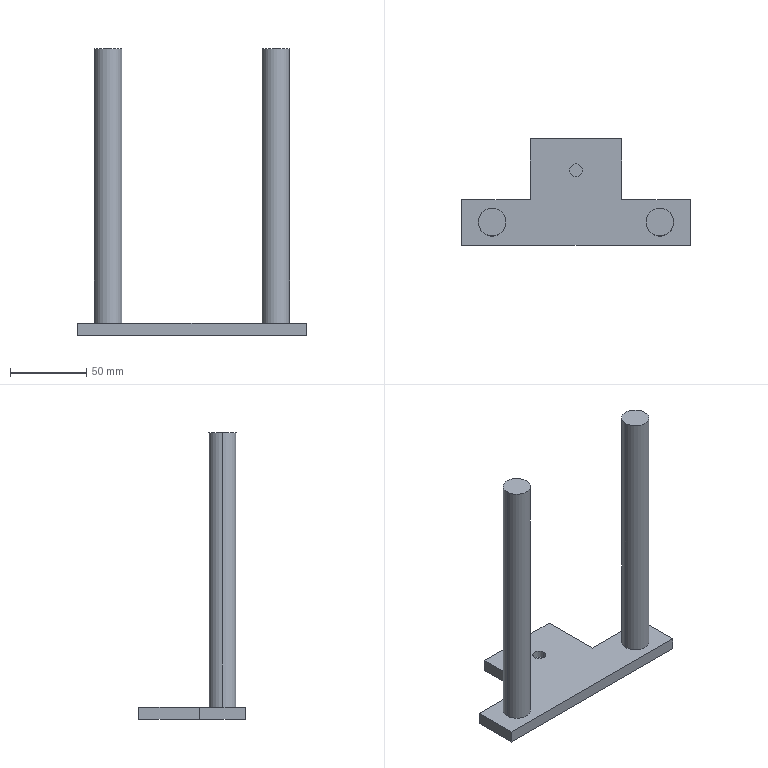Part | STEP file | 1 solid | 19 faces | box 150 x 70 x 188 mm | volume 146525 mm3 | plane 13 | cylinder 6 | commonest cylinder face diameters 18 x4 8.5 x2
STEP:
#1=CARTESIAN_POINT('',(0.,0.,0.));
#2=DIRECTION('',(0.,0.,1.));
#3=DIRECTION('',(1.,0.,0.));
#4=AXIS2_PLACEMENT_3D('',#1,#2,#3);
#5=CARTESIAN_POINT('',(-46.,15.,8.));
#6=VERTEX_POINT('',#5);
#7=CARTESIAN_POINT('',(-64.,15.,8.));
#8=VERTEX_POINT('',#7);
#9=CARTESIAN_POINT('',(-55.,15.,8.));
#10=DIRECTION('',(0.,0.,1.));
#11=DIRECTION('',(1.,0.,0.));
#12=AXIS2_PLACEMENT_3D('',#9,#10,#11);
#13=CIRCLE('',#12,9.);
#14=CARTESIAN_POINT('',(-55.,15.,188.));
#15=DIRECTION('',(0.,0.,1.));
#16=DIRECTION('',(1.,0.,0.));
#17=AXIS2_PLACEMENT_3D('',#14,#15,#16);
#18=CYLINDRICAL_SURFACE('',#17,9.);
#19=CARTESIAN_POINT('',(0.,-180.));
#20=DIRECTION('',(1.,0.));
#21=VECTOR('',#20,1.);
#22=LINE('',#19,#21);
#23=(GEOMETRIC_REPRESENTATION_CONTEXT(2)PARAMETRIC_REPRESENTATION_CONTEXT()REPRESENTATION_CONTEXT('',''));
#24=DEFINITIONAL_REPRESENTATION('',(#22),#23);
#25=PCURVE('',#18,#24);
#26=CARTESIAN_POINT('',(0.,0.,8.));
#27=DIRECTION('',(0.,0.,-1.));
#28=DIRECTION('',(-1.,0.,0.));
#29=AXIS2_PLACEMENT_3D('',#26,#27,#28);
#30=PLANE('',#29);
#31=CARTESIAN_POINT('',(46.,15.));
#32=CARTESIAN_POINT('',(46.,30.588));
#33=CARTESIAN_POINT('',(59.5,22.794));
#34=CARTESIAN_POINT('',(73.,15.));
#35=CARTESIAN_POINT('',(59.5,7.206));
#36=CARTESIAN_POINT('',(46.,-0.5885));
#37=CARTESIAN_POINT('',(46.,15.));
#38=(BOUNDED_CURVE()B_SPLINE_CURVE(2,(#31,#32,#33,#34,#35,#36,#37),.UNSPECIFIED.,.T.,.F.)B_SPLINE_CURVE_WITH_KNOTS((1,2,2,2,2,1),(-2.094,0.,2.094,4.189,6.283,8.378),.UNSPECIFIED.)CURVE()GEOMETRIC_REPRESENTATION_ITEM()RATIONAL_B_SPLINE_CURVE((1.,0.5,1.,0.5,1.,0.5,1.))REPRESENTATION_ITEM(''));
#39=(GEOMETRIC_REPRESENTATION_CONTEXT(2)PARAMETRIC_REPRESENTATION_CONTEXT()REPRESENTATION_CONTEXT('',''));
#40=DEFINITIONAL_REPRESENTATION('',(#38),#39);
#41=PCURVE('',#30,#40);
#42=SURFACE_CURVE('',#13,(#25,#41),.PCURVE_S1.);
#43=EDGE_CURVE('',#6,#8,#42,.T.);
#44=ORIENTED_EDGE('',*,*,#43,.T.);
#45=CARTESIAN_POINT('',(-64.,15.,188.));
#46=VERTEX_POINT('',#45);
#47=CARTESIAN_POINT('',(-64.,15.,188.));
#48=DIRECTION('',(0.,0.,1.));
#49=VECTOR('',#48,1.);
#50=LINE('',#47,#49);
#51=CARTESIAN_POINT('',(3.142,0.));
#52=DIRECTION('',(0.,1.));
#53=VECTOR('',#52,1.);
#54=LINE('',#51,#53);
#55=(GEOMETRIC_REPRESENTATION_CONTEXT(2)PARAMETRIC_REPRESENTATION_CONTEXT()REPRESENTATION_CONTEXT('',''));
#56=DEFINITIONAL_REPRESENTATION('',(#54),#55);
#57=PCURVE('',#18,#56);
#58=CARTESIAN_POINT('',(-55.,15.,188.));
#59=DIRECTION('',(0.,0.,1.));
#60=DIRECTION('',(1.,0.,0.));
#61=AXIS2_PLACEMENT_3D('',#58,#59,#60);
#62=CYLINDRICAL_SURFACE('',#61,9.);
#63=CARTESIAN_POINT('',(3.142,0.));
#64=DIRECTION('',(0.,1.));
#65=VECTOR('',#64,1.);
#66=LINE('',#63,#65);
#67=(GEOMETRIC_REPRESENTATION_CONTEXT(2)PARAMETRIC_REPRESENTATION_CONTEXT()REPRESENTATION_CONTEXT('',''));
#68=DEFINITIONAL_REPRESENTATION('',(#66),#67);
#69=PCURVE('',#62,#68);
#70=SURFACE_CURVE('',#50,(#57,#69),.PCURVE_S1.);
#71=EDGE_CURVE('',#8,#46,#70,.T.);
#72=ORIENTED_EDGE('',*,*,#71,.T.);
#73=CARTESIAN_POINT('',(-46.,15.,188.));
#74=VERTEX_POINT('',#73);
#75=CARTESIAN_POINT('',(-55.,15.,188.));
#76=DIRECTION('',(0.,0.,-1.));
#77=DIRECTION('',(1.,0.,0.));
#78=AXIS2_PLACEMENT_3D('',#75,#76,#77);
#79=CIRCLE('',#78,9.);
#80=CARTESIAN_POINT('',(6.283,0.));
#81=DIRECTION('',(-1.,0.));
#82=VECTOR('',#81,1.);
#83=LINE('',#80,#82);
#84=(GEOMETRIC_REPRESENTATION_CONTEXT(2)PARAMETRIC_REPRESENTATION_CONTEXT()REPRESENTATION_CONTEXT('',''));
#85=DEFINITIONAL_REPRESENTATION('',(#83),#84);
#86=PCURVE('',#18,#85);
#87=CARTESIAN_POINT('',(-55.,15.,188.));
#88=DIRECTION('',(0.,0.,1.));
#89=DIRECTION('',(1.,0.,0.));
#90=AXIS2_PLACEMENT_3D('',#87,#88,#89);
#91=PLANE('',#90);
#92=CARTESIAN_POINT('',(9.,0.));
#93=CARTESIAN_POINT('',(9.,-15.588));
#94=CARTESIAN_POINT('',(-4.5,-7.794));
#95=CARTESIAN_POINT('',(-18.,0.));
#96=CARTESIAN_POINT('',(-4.5,7.794));
#97=CARTESIAN_POINT('',(9.,15.588));
#98=CARTESIAN_POINT('',(9.,0.));
#99=(BOUNDED_CURVE()B_SPLINE_CURVE(2,(#92,#93,#94,#95,#96,#97,#98),.UNSPECIFIED.,.T.,.F.)B_SPLINE_CURVE_WITH_KNOTS((1,2,2,2,2,1),(-2.094,0.,2.094,4.189,6.283,8.378),.UNSPECIFIED.)CURVE()GEOMETRIC_REPRESENTATION_ITEM()RATIONAL_B_SPLINE_CURVE((1.,0.5,1.,0.5,1.,0.5,1.))REPRESENTATION_ITEM(''));
#100=(GEOMETRIC_REPRESENTATION_CONTEXT(2)PARAMETRIC_REPRESENTATION_CONTEXT()REPRESENTATION_CONTEXT('',''));
#101=DEFINITIONAL_REPRESENTATION('',(#99),#100);
#102=PCURVE('',#91,#101);
#103=SURFACE_CURVE('',#79,(#86,#102),.PCURVE_S1.);
#104=EDGE_CURVE('',#46,#74,#103,.T.);
#105=ORIENTED_EDGE('',*,*,#104,.T.);
#106=CARTESIAN_POINT('',(-46.,15.,188.));
#107=DIRECTION('',(0.,0.,1.));
#108=VECTOR('',#107,1.);
#109=LINE('',#106,#108);
#110=CARTESIAN_POINT('',(0.,0.));
#111=DIRECTION('',(0.,1.));
#112=VECTOR('',#111,1.);
#113=LINE('',#110,#112);
#114=(GEOMETRIC_REPRESENTATION_CONTEXT(2)PARAMETRIC_REPRESENTATION_CONTEXT()REPRESENTATION_CONTEXT('',''));
#115=DEFINITIONAL_REPRESENTATION('',(#113),#114);
#116=PCURVE('',#18,#115);
#117=CARTESIAN_POINT('',(6.283,0.));
#118=DIRECTION('',(0.,1.));
#119=VECTOR('',#118,1.);
#120=LINE('',#117,#119);
#121=(GEOMETRIC_REPRESENTATION_CONTEXT(2)PARAMETRIC_REPRESENTATION_CONTEXT()REPRESENTATION_CONTEXT('',''));
#122=DEFINITIONAL_REPRESENTATION('',(#120),#121);
#123=PCURVE('',#62,#122);
#124=SURFACE_CURVE('',#109,(#116,#123),.PCURVE_S1.);
#125=EDGE_CURVE('',#6,#74,#124,.T.);
#126=ORIENTED_EDGE('',*,*,#125,.F.);
#127=EDGE_LOOP('',(#44,#72,#105,#126));
#128=FACE_BOUND('',#127,.T.);
#129=ADVANCED_FACE('',(#128),#18,.T.);
#130=CARTESIAN_POINT('',(64.,15.,8.));
#131=VERTEX_POINT('',#130);
#132=CARTESIAN_POINT('',(46.,15.,8.));
#133=VERTEX_POINT('',#132);
#134=CARTESIAN_POINT('',(55.,15.,8.));
#135=DIRECTION('',(0.,0.,1.));
#136=DIRECTION('',(1.,0.,0.));
#137=AXIS2_PLACEMENT_3D('',#134,#135,#136);
#138=CIRCLE('',#137,9.);
#139=CARTESIAN_POINT('',(55.,15.,188.));
#140=DIRECTION('',(0.,0.,1.));
#141=DIRECTION('',(1.,0.,0.));
#142=AXIS2_PLACEMENT_3D('',#139,#140,#141);
#143=CYLINDRICAL_SURFACE('',#142,9.);
#144=CARTESIAN_POINT('',(0.,-180.));
#145=DIRECTION('',(1.,0.));
#146=VECTOR('',#145,1.);
#147=LINE('',#144,#146);
#148=(GEOMETRIC_REPRESENTATION_CONTEXT(2)PARAMETRIC_REPRESENTATION_CONTEXT()REPRESENTATION_CONTEXT('',''));
#149=DEFINITIONAL_REPRESENTATION('',(#147),#148);
#150=PCURVE('',#143,#149);
#151=CARTESIAN_POINT('',(-64.,15.));
#152=CARTESIAN_POINT('',(-64.,30.588));
#153=CARTESIAN_POINT('',(-50.5,22.794));
#154=CARTESIAN_POINT('',(-37.,15.));
#155=CARTESIAN_POINT('',(-50.5,7.206));
#156=CARTESIAN_POINT('',(-64.,-0.5885));
#157=CARTESIAN_POINT('',(-64.,15.));
#158=(BOUNDED_CURVE()B_SPLINE_CURVE(2,(#151,#152,#153,#154,#155,#156,#157),.UNSPECIFIED.,.T.,.F.)B_SPLINE_CURVE_WITH_KNOTS((1,2,2,2,2,1),(-2.094,0.,2.094,4.189,6.283,8.378),.UNSPECIFIED.)CURVE()GEOMETRIC_REPRESENTATION_ITEM()RATIONAL_B_SPLINE_CURVE((1.,0.5,1.,0.5,1.,0.5,1.))REPRESENTATION_ITEM(''));
#159=(GEOMETRIC_REPRESENTATION_CONTEXT(2)PARAMETRIC_REPRESENTATION_CONTEXT()REPRESENTATION_CONTEXT('',''));
#160=DEFINITIONAL_REPRESENTATION('',(#158),#159);
#161=PCURVE('',#30,#160);
#162=SURFACE_CURVE('',#138,(#150,#161),.PCURVE_S1.);
#163=EDGE_CURVE('',#131,#133,#162,.T.);
#164=ORIENTED_EDGE('',*,*,#163,.T.);
#165=CARTESIAN_POINT('',(46.,15.,188.));
#166=VERTEX_POINT('',#165);
#167=CARTESIAN_POINT('',(46.,15.,188.));
#168=DIRECTION('',(0.,0.,1.));
#169=VECTOR('',#168,1.);
#170=LINE('',#167,#169);
#171=CARTESIAN_POINT('',(3.142,0.));
#172=DIRECTION('',(0.,1.));
#173=VECTOR('',#172,1.);
#174=LINE('',#171,#173);
#175=(GEOMETRIC_REPRESENTATION_CONTEXT(2)PARAMETRIC_REPRESENTATION_CONTEXT()REPRESENTATION_CONTEXT('',''));
#176=DEFINITIONAL_REPRESENTATION('',(#174),#175);
#177=PCURVE('',#143,#176);
#178=CARTESIAN_POINT('',(55.,15.,188.));
#179=DIRECTION('',(0.,0.,1.));
#180=DIRECTION('',(1.,0.,0.));
#181=AXIS2_PLACEMENT_3D('',#178,#179,#180);
#182=CYLINDRICAL_SURFACE('',#181,9.);
#183=CARTESIAN_POINT('',(3.142,0.));
#184=DIRECTION('',(0.,1.));
#185=VECTOR('',#184,1.);
#186=LINE('',#183,#185);
#187=(GEOMETRIC_REPRESENTATION_CONTEXT(2)PARAMETRIC_REPRESENTATION_CONTEXT()REPRESENTATION_CONTEXT('',''));
#188=DEFINITIONAL_REPRESENTATION('',(#186),#187);
#189=PCURVE('',#182,#188);
#190=SURFACE_CURVE('',#170,(#177,#189),.PCURVE_S1.);
#191=EDGE_CURVE('',#133,#166,#190,.T.);
#192=ORIENTED_EDGE('',*,*,#191,.T.);
#193=CARTESIAN_POINT('',(64.,15.,188.));
#194=VERTEX_POINT('',#193);
#195=CARTESIAN_POINT('',(55.,15.,188.));
#196=DIRECTION('',(0.,0.,-1.));
#197=DIRECTION('',(1.,0.,0.));
#198=AXIS2_PLACEMENT_3D('',#195,#196,#197);
#199=CIRCLE('',#198,9.);
#200=CARTESIAN_POINT('',(6.283,0.));
#201=DIRECTION('',(-1.,0.));
#202=VECTOR('',#201,1.);
#203=LINE('',#200,#202);
#204=(GEOMETRIC_REPRESENTATION_CONTEXT(2)PARAMETRIC_REPRESENTATION_CONTEXT()REPRESENTATION_CONTEXT('',''));
#205=DEFINITIONAL_REPRESENTATION('',(#203),#204);
#206=PCURVE('',#143,#205);
#207=CARTESIAN_POINT('',(55.,15.,188.));
#208=DIRECTION('',(0.,0.,-1.));
#209=DIRECTION('',(-1.,0.,0.));
#210=AXIS2_PLACEMENT_3D('',#207,#208,#209);
#211=PLANE('',#210);
#212=CARTESIAN_POINT('',(0.,0.));
#213=DIRECTION('',(-1.,0.));
#214=AXIS2_PLACEMENT_2D('',#212,#213);
#215=CIRCLE('',#214,9.);
#216=(GEOMETRIC_REPRESENTATION_CONTEXT(2)PARAMETRIC_REPRESENTATION_CONTEXT()REPRESENTATION_CONTEXT('',''));
#217=DEFINITIONAL_REPRESENTATION('',(#215),#216);
#218=PCURVE('',#211,#217);
#219=SURFACE_CURVE('',#199,(#206,#218),.PCURVE_S1.);
#220=EDGE_CURVE('',#166,#194,#219,.T.);
#221=ORIENTED_EDGE('',*,*,#220,.T.);
#222=CARTESIAN_POINT('',(64.,15.,188.));
#223=DIRECTION('',(0.,0.,1.));
#224=VECTOR('',#223,1.);
#225=LINE('',#222,#224);
#226=CARTESIAN_POINT('',(0.,0.));
#227=DIRECTION('',(0.,1.));
#228=VECTOR('',#227,1.);
#229=LINE('',#226,#228);
#230=(GEOMETRIC_REPRESENTATION_CONTEXT(2)PARAMETRIC_REPRESENTATION_CONTEXT()REPRESENTATION_CONTEXT('',''));
#231=DEFINITIONAL_REPRESENTATION('',(#229),#230);
#232=PCURVE('',#143,#231);
#233=CARTESIAN_POINT('',(6.283,0.));
#234=DIRECTION('',(0.,1.));
#235=VECTOR('',#234,1.);
#236=LINE('',#233,#235);
#237=(GEOMETRIC_REPRESENTATION_CONTEXT(2)PARAMETRIC_REPRESENTATION_CONTEXT()REPRESENTATION_CONTEXT('',''));
#238=DEFINITIONAL_REPRESENTATION('',(#236),#237);
#239=PCURVE('',#182,#238);
#240=SURFACE_CURVE('',#225,(#232,#239),.PCURVE_S1.);
#241=EDGE_CURVE('',#131,#194,#240,.T.);
#242=ORIENTED_EDGE('',*,*,#241,.F.);
#243=EDGE_LOOP('',(#164,#192,#221,#242));
#244=FACE_BOUND('',#243,.T.);
#245=ADVANCED_FACE('',(#244),#143,.T.);
#246=CARTESIAN_POINT('',(-4.25,49.16,8.));
#247=VERTEX_POINT('',#246);
#248=CARTESIAN_POINT('',(-4.25,49.16,3.));
#249=VERTEX_POINT('',#248);
#250=CARTESIAN_POINT('',(-4.25,49.16,3.));
#251=DIRECTION('',(0.,0.,-1.));
#252=VECTOR('',#251,1.);
#253=LINE('',#250,#252);
#254=CARTESIAN_POINT('',(0.,49.16,3.));
#255=DIRECTION('',(0.,0.,-1.));
#256=DIRECTION('',(-1.,0.,0.));
#257=AXIS2_PLACEMENT_3D('',#254,#255,#256);
#258=CYLINDRICAL_SURFACE('',#257,4.25);
#259=CARTESIAN_POINT('',(6.283,0.));
#260=DIRECTION('',(0.,1.));
#261=VECTOR('',#260,1.);
#262=LINE('',#259,#261);
#263=(GEOMETRIC_REPRESENTATION_CONTEXT(2)PARAMETRIC_REPRESENTATION_CONTEXT()REPRESENTATION_CONTEXT('',''));
#264=DEFINITIONAL_REPRESENTATION('',(#262),#263);
#265=PCURVE('',#258,#264);
#266=CARTESIAN_POINT('',(0.,49.16,3.));
#267=DIRECTION('',(0.,0.,-1.));
#268=DIRECTION('',(-1.,0.,0.));
#269=AXIS2_PLACEMENT_3D('',#266,#267,#268);
#270=CYLINDRICAL_SURFACE('',#269,4.25);
#271=CARTESIAN_POINT('',(0.,0.));
#272=DIRECTION('',(0.,1.));
#273=VECTOR('',#272,1.);
#274=LINE('',#271,#273);
#275=(GEOMETRIC_REPRESENTATION_CONTEXT(2)PARAMETRIC_REPRESENTATION_CONTEXT()REPRESENTATION_CONTEXT('',''));
#276=DEFINITIONAL_REPRESENTATION('',(#274),#275);
#277=PCURVE('',#270,#276);
#278=SURFACE_CURVE('',#253,(#265,#277),.PCURVE_S1.);
#279=EDGE_CURVE('',#247,#249,#278,.T.);
#280=ORIENTED_EDGE('',*,*,#279,.T.);
#281=CARTESIAN_POINT('',(4.25,49.16,3.));
#282=VERTEX_POINT('',#281);
#283=CARTESIAN_POINT('',(0.,49.16,3.));
#284=DIRECTION('',(0.,0.,1.));
#285=DIRECTION('',(-1.,0.,0.));
#286=AXIS2_PLACEMENT_3D('',#283,#284,#285);
#287=CIRCLE('',#286,4.25);
#288=CARTESIAN_POINT('',(6.283,0.));
#289=DIRECTION('',(-1.,0.));
#290=VECTOR('',#289,1.);
#291=LINE('',#288,#290);
#292=(GEOMETRIC_REPRESENTATION_CONTEXT(2)PARAMETRIC_REPRESENTATION_CONTEXT()REPRESENTATION_CONTEXT('',''));
#293=DEFINITIONAL_REPRESENTATION('',(#291),#292);
#294=PCURVE('',#258,#293);
#295=CARTESIAN_POINT('',(0.,49.16,3.));
#296=DIRECTION('',(0.,0.,1.));
#297=DIRECTION('',(1.,0.,0.));
#298=AXIS2_PLACEMENT_3D('',#295,#296,#297);
#299=PLANE('',#298);
#300=CARTESIAN_POINT('',(0.,0.));
#301=DIRECTION('',(-1.,0.));
#302=AXIS2_PLACEMENT_2D('',#300,#301);
#303=CIRCLE('',#302,4.25);
#304=(GEOMETRIC_REPRESENTATION_CONTEXT(2)PARAMETRIC_REPRESENTATION_CONTEXT()REPRESENTATION_CONTEXT('',''));
#305=DEFINITIONAL_REPRESENTATION('',(#303),#304);
#306=PCURVE('',#299,#305);
#307=SURFACE_CURVE('',#287,(#294,#306),.PCURVE_S1.);
#308=EDGE_CURVE('',#249,#282,#307,.T.);
#309=ORIENTED_EDGE('',*,*,#308,.T.);
#310=CARTESIAN_POINT('',(4.25,49.16,8.));
#311=VERTEX_POINT('',#310);
#312=CARTESIAN_POINT('',(4.25,49.16,3.));
#313=DIRECTION('',(0.,0.,-1.));
#314=VECTOR('',#313,1.);
#315=LINE('',#312,#314);
#316=CARTESIAN_POINT('',(3.142,0.));
#317=DIRECTION('',(0.,1.));
#318=VECTOR('',#317,1.);
#319=LINE('',#316,#318);
#320=(GEOMETRIC_REPRESENTATION_CONTEXT(2)PARAMETRIC_REPRESENTATION_CONTEXT()REPRESENTATION_CONTEXT('',''));
#321=DEFINITIONAL_REPRESENTATION('',(#319),#320);
#322=PCURVE('',#258,#321);
#323=CARTESIAN_POINT('',(3.142,0.));
#324=DIRECTION('',(0.,1.));
#325=VECTOR('',#324,1.);
#326=LINE('',#323,#325);
#327=(GEOMETRIC_REPRESENTATION_CONTEXT(2)PARAMETRIC_REPRESENTATION_CONTEXT()REPRESENTATION_CONTEXT('',''));
#328=DEFINITIONAL_REPRESENTATION('',(#326),#327);
#329=PCURVE('',#270,#328);
#330=SURFACE_CURVE('',#315,(#322,#329),.PCURVE_S1.);
#331=EDGE_CURVE('',#311,#282,#330,.T.);
#332=ORIENTED_EDGE('',*,*,#331,.F.);
#333=CARTESIAN_POINT('',(0.,49.16,8.));
#334=DIRECTION('',(0.,0.,1.));
#335=DIRECTION('',(-1.,0.,0.));
#336=AXIS2_PLACEMENT_3D('',#333,#334,#335);
#337=CIRCLE('',#336,4.25);
#338=CARTESIAN_POINT('',(6.283,-5.));
#339=DIRECTION('',(-1.,0.));
#340=VECTOR('',#339,1.);
#341=LINE('',#338,#340);
#342=(GEOMETRIC_REPRESENTATION_CONTEXT(2)PARAMETRIC_REPRESENTATION_CONTEXT()REPRESENTATION_CONTEXT('',''));
#343=DEFINITIONAL_REPRESENTATION('',(#341),#342);
#344=PCURVE('',#258,#343);
#345=CARTESIAN_POINT('',(4.25,49.16));
#346=CARTESIAN_POINT('',(4.25,41.799));
#347=CARTESIAN_POINT('',(-2.125,45.48));
#348=CARTESIAN_POINT('',(-8.5,49.16));
#349=CARTESIAN_POINT('',(-2.125,52.84));
#350=CARTESIAN_POINT('',(4.25,56.521));
#351=CARTESIAN_POINT('',(4.25,49.16));
#352=(BOUNDED_CURVE()B_SPLINE_CURVE(2,(#345,#346,#347,#348,#349,#350,#351),.UNSPECIFIED.,.T.,.F.)B_SPLINE_CURVE_WITH_KNOTS((1,2,2,2,2,1),(-2.094,0.,2.094,4.189,6.283,8.378),.UNSPECIFIED.)CURVE()GEOMETRIC_REPRESENTATION_ITEM()RATIONAL_B_SPLINE_CURVE((1.,0.5,1.,0.5,1.,0.5,1.))REPRESENTATION_ITEM(''));
#353=(GEOMETRIC_REPRESENTATION_CONTEXT(2)PARAMETRIC_REPRESENTATION_CONTEXT()REPRESENTATION_CONTEXT('',''));
#354=DEFINITIONAL_REPRESENTATION('',(#352),#353);
#355=PCURVE('',#30,#354);
#356=SURFACE_CURVE('',#337,(#344,#355),.PCURVE_S1.);
#357=EDGE_CURVE('',#247,#311,#356,.T.);
#358=ORIENTED_EDGE('',*,*,#357,.F.);
#359=EDGE_LOOP('',(#280,#309,#332,#358));
#360=FACE_BOUND('',#359,.F.);
#361=ADVANCED_FACE('',(#360),#258,.F.);
#362=CARTESIAN_POINT('',(-75.,0.,0.));
#363=VERTEX_POINT('',#362);
#364=CARTESIAN_POINT('',(-75.,30.,0.));
#365=VERTEX_POINT('',#364);
#366=CARTESIAN_POINT('',(-75.,0.,0.));
#367=DIRECTION('',(0.,1.,0.));
#368=VECTOR('',#367,1.);
#369=LINE('',#366,#368);
#370=CARTESIAN_POINT('',(0.,0.,0.));
#371=DIRECTION('',(0.,0.,-1.));
#372=DIRECTION('',(-1.,0.,0.));
#373=AXIS2_PLACEMENT_3D('',#370,#371,#372);
#374=PLANE('',#373);
#375=CARTESIAN_POINT('',(75.,0.));
#376=DIRECTION('',(0.,1.));
#377=VECTOR('',#376,1.);
#378=LINE('',#375,#377);
#379=(GEOMETRIC_REPRESENTATION_CONTEXT(2)PARAMETRIC_REPRESENTATION_CONTEXT()REPRESENTATION_CONTEXT('',''));
#380=DEFINITIONAL_REPRESENTATION('',(#378),#379);
#381=PCURVE('',#374,#380);
#382=CARTESIAN_POINT('',(-75.,0.,8.));
#383=DIRECTION('',(1.,0.,0.));
#384=DIRECTION('',(0.,0.,-1.));
#385=AXIS2_PLACEMENT_3D('',#382,#383,#384);
#386=PLANE('',#385);
#387=CARTESIAN_POINT('',(8.,0.));
#388=DIRECTION('',(0.,1.));
#389=VECTOR('',#388,1.);
#390=LINE('',#387,#389);
#391=(GEOMETRIC_REPRESENTATION_CONTEXT(2)PARAMETRIC_REPRESENTATION_CONTEXT()REPRESENTATION_CONTEXT('',''));
#392=DEFINITIONAL_REPRESENTATION('',(#390),#391);
#393=PCURVE('',#386,#392);
#394=SURFACE_CURVE('',#369,(#381,#393),.PCURVE_S1.);
#395=EDGE_CURVE('',#363,#365,#394,.T.);
#396=ORIENTED_EDGE('',*,*,#395,.T.);
#397=CARTESIAN_POINT('',(-30.,30.,0.));
#398=VERTEX_POINT('',#397);
#399=CARTESIAN_POINT('',(0.,30.,0.));
#400=DIRECTION('',(1.,0.,0.));
#401=VECTOR('',#400,1.);
#402=LINE('',#399,#401);
#403=CARTESIAN_POINT('',(0.,30.));
#404=DIRECTION('',(-1.,0.));
#405=VECTOR('',#404,1.);
#406=LINE('',#403,#405);
#407=(GEOMETRIC_REPRESENTATION_CONTEXT(2)PARAMETRIC_REPRESENTATION_CONTEXT()REPRESENTATION_CONTEXT('',''));
#408=DEFINITIONAL_REPRESENTATION('',(#406),#407);
#409=PCURVE('',#374,#408);
#410=CARTESIAN_POINT('',(-75.,30.,8.));
#411=DIRECTION('',(0.,-1.,0.));
#412=DIRECTION('',(0.,0.,-1.));
#413=AXIS2_PLACEMENT_3D('',#410,#411,#412);
#414=PLANE('',#413);
#415=CARTESIAN_POINT('',(8.,75.));
#416=DIRECTION('',(0.,1.));
#417=VECTOR('',#416,1.);
#418=LINE('',#415,#417);
#419=(GEOMETRIC_REPRESENTATION_CONTEXT(2)PARAMETRIC_REPRESENTATION_CONTEXT()REPRESENTATION_CONTEXT('',''));
#420=DEFINITIONAL_REPRESENTATION('',(#418),#419);
#421=PCURVE('',#414,#420);
#422=SURFACE_CURVE('',#402,(#409,#421),.PCURVE_S1.);
#423=EDGE_CURVE('',#365,#398,#422,.T.);
#424=ORIENTED_EDGE('',*,*,#423,.T.);
#425=CARTESIAN_POINT('',(-30.,70.,0.));
#426=VERTEX_POINT('',#425);
#427=CARTESIAN_POINT('',(-30.,0.,0.));
#428=DIRECTION('',(0.,1.,0.));
#429=VECTOR('',#428,1.);
#430=LINE('',#427,#429);
#431=CARTESIAN_POINT('',(30.,0.));
#432=DIRECTION('',(0.,1.));
#433=VECTOR('',#432,1.);
#434=LINE('',#431,#433);
#435=(GEOMETRIC_REPRESENTATION_CONTEXT(2)PARAMETRIC_REPRESENTATION_CONTEXT()REPRESENTATION_CONTEXT('',''));
#436=DEFINITIONAL_REPRESENTATION('',(#434),#435);
#437=PCURVE('',#374,#436);
#438=CARTESIAN_POINT('',(-30.,30.,8.));
#439=DIRECTION('',(1.,0.,0.));
#440=DIRECTION('',(0.,0.,-1.));
#441=AXIS2_PLACEMENT_3D('',#438,#439,#440);
#442=PLANE('',#441);
#443=CARTESIAN_POINT('',(8.,-30.));
#444=DIRECTION('',(0.,1.));
#445=VECTOR('',#444,1.);
#446=LINE('',#443,#445);
#447=(GEOMETRIC_REPRESENTATION_CONTEXT(2)PARAMETRIC_REPRESENTATION_CONTEXT()REPRESENTATION_CONTEXT('',''));
#448=DEFINITIONAL_REPRESENTATION('',(#446),#447);
#449=PCURVE('',#442,#448);
#450=SURFACE_CURVE('',#430,(#437,#449),.PCURVE_S1.);
#451=EDGE_CURVE('',#398,#426,#450,.T.);
#452=ORIENTED_EDGE('',*,*,#451,.T.);
#453=CARTESIAN_POINT('',(30.,70.,0.));
#454=VERTEX_POINT('',#453);
#455=CARTESIAN_POINT('',(0.,70.,0.));
#456=DIRECTION('',(1.,0.,0.));
#457=VECTOR('',#456,1.);
#458=LINE('',#455,#457);
#459=CARTESIAN_POINT('',(0.,70.));
#460=DIRECTION('',(-1.,0.));
#461=VECTOR('',#460,1.);
#462=LINE('',#459,#461);
#463=(GEOMETRIC_REPRESENTATION_CONTEXT(2)PARAMETRIC_REPRESENTATION_CONTEXT()REPRESENTATION_CONTEXT('',''));
#464=DEFINITIONAL_REPRESENTATION('',(#462),#463);
#465=PCURVE('',#374,#464);
#466=CARTESIAN_POINT('',(-30.,70.,8.));
#467=DIRECTION('',(0.,-1.,0.));
#468=DIRECTION('',(1.,0.,0.));
#469=AXIS2_PLACEMENT_3D('',#466,#467,#468);
#470=PLANE('',#469);
#471=CARTESIAN_POINT('',(30.,-8.));
#472=DIRECTION('',(1.,0.));
#473=VECTOR('',#472,1.);
#474=LINE('',#471,#473);
#475=(GEOMETRIC_REPRESENTATION_CONTEXT(2)PARAMETRIC_REPRESENTATION_CONTEXT()REPRESENTATION_CONTEXT('',''));
#476=DEFINITIONAL_REPRESENTATION('',(#474),#475);
#477=PCURVE('',#470,#476);
#478=SURFACE_CURVE('',#458,(#465,#477),.PCURVE_S1.);
#479=EDGE_CURVE('',#426,#454,#478,.T.);
#480=ORIENTED_EDGE('',*,*,#479,.T.);
#481=CARTESIAN_POINT('',(30.,30.,0.));
#482=VERTEX_POINT('',#481);
#483=CARTESIAN_POINT('',(30.,0.,0.));
#484=DIRECTION('',(0.,-1.,0.));
#485=VECTOR('',#484,1.);
#486=LINE('',#483,#485);
#487=CARTESIAN_POINT('',(-30.,0.));
#488=DIRECTION('',(0.,-1.));
#489=VECTOR('',#488,1.);
#490=LINE('',#487,#489);
#491=(GEOMETRIC_REPRESENTATION_CONTEXT(2)PARAMETRIC_REPRESENTATION_CONTEXT()REPRESENTATION_CONTEXT('',''));
#492=DEFINITIONAL_REPRESENTATION('',(#490),#491);
#493=PCURVE('',#374,#492);
#494=CARTESIAN_POINT('',(30.,30.,8.));
#495=DIRECTION('',(-1.,0.,0.));
#496=DIRECTION('',(0.,-1.,0.));
#497=AXIS2_PLACEMENT_3D('',#494,#495,#496);
#498=PLANE('',#497);
#499=CARTESIAN_POINT('',(30.,-8.));
#500=DIRECTION('',(1.,0.));
#501=VECTOR('',#500,1.);
#502=LINE('',#499,#501);
#503=(GEOMETRIC_REPRESENTATION_CONTEXT(2)PARAMETRIC_REPRESENTATION_CONTEXT()REPRESENTATION_CONTEXT('',''));
#504=DEFINITIONAL_REPRESENTATION('',(#502),#503);
#505=PCURVE('',#498,#504);
#506=SURFACE_CURVE('',#486,(#493,#505),.PCURVE_S1.);
#507=EDGE_CURVE('',#454,#482,#506,.T.);
#508=ORIENTED_EDGE('',*,*,#507,.T.);
#509=CARTESIAN_POINT('',(75.,30.,0.));
#510=VERTEX_POINT('',#509);
#511=CARTESIAN_POINT('',(0.,30.,0.));
#512=DIRECTION('',(1.,0.,0.));
#513=VECTOR('',#512,1.);
#514=LINE('',#511,#513);
#515=CARTESIAN_POINT('',(0.,30.));
#516=DIRECTION('',(-1.,0.));
#517=VECTOR('',#516,1.);
#518=LINE('',#515,#517);
#519=(GEOMETRIC_REPRESENTATION_CONTEXT(2)PARAMETRIC_REPRESENTATION_CONTEXT()REPRESENTATION_CONTEXT('',''));
#520=DEFINITIONAL_REPRESENTATION('',(#518),#519);
#521=PCURVE('',#374,#520);
#522=CARTESIAN_POINT('',(75.,30.,8.));
#523=DIRECTION('',(0.,-1.,0.));
#524=DIRECTION('',(1.,0.,0.));
#525=AXIS2_PLACEMENT_3D('',#522,#523,#524);
#526=PLANE('',#525);
#527=CARTESIAN_POINT('',(-75.,-8.));
#528=DIRECTION('',(1.,0.));
#529=VECTOR('',#528,1.);
#530=LINE('',#527,#529);
#531=(GEOMETRIC_REPRESENTATION_CONTEXT(2)PARAMETRIC_REPRESENTATION_CONTEXT()REPRESENTATION_CONTEXT('',''));
#532=DEFINITIONAL_REPRESENTATION('',(#530),#531);
#533=PCURVE('',#526,#532);
#534=SURFACE_CURVE('',#514,(#521,#533),.PCURVE_S1.);
#535=EDGE_CURVE('',#482,#510,#534,.T.);
#536=ORIENTED_EDGE('',*,*,#535,.T.);
#537=CARTESIAN_POINT('',(75.,0.,0.));
#538=VERTEX_POINT('',#537);
#539=CARTESIAN_POINT('',(75.,0.,0.));
#540=DIRECTION('',(0.,-1.,0.));
#541=VECTOR('',#540,1.);
#542=LINE('',#539,#541);
#543=CARTESIAN_POINT('',(-75.,0.));
#544=DIRECTION('',(0.,-1.));
#545=VECTOR('',#544,1.);
#546=LINE('',#543,#545);
#547=(GEOMETRIC_REPRESENTATION_CONTEXT(2)PARAMETRIC_REPRESENTATION_CONTEXT()REPRESENTATION_CONTEXT('',''));
#548=DEFINITIONAL_REPRESENTATION('',(#546),#547);
#549=PCURVE('',#374,#548);
#550=CARTESIAN_POINT('',(75.,0.,8.));
#551=DIRECTION('',(-1.,0.,0.));
#552=DIRECTION('',(0.,0.,1.));
#553=AXIS2_PLACEMENT_3D('',#550,#551,#552);
#554=PLANE('',#553);
#555=CARTESIAN_POINT('',(-8.,0.));
#556=DIRECTION('',(0.,-1.));
#557=VECTOR('',#556,1.);
#558=LINE('',#555,#557);
#559=(GEOMETRIC_REPRESENTATION_CONTEXT(2)PARAMETRIC_REPRESENTATION_CONTEXT()REPRESENTATION_CONTEXT('',''));
#560=DEFINITIONAL_REPRESENTATION('',(#558),#559);
#561=PCURVE('',#554,#560);
#562=SURFACE_CURVE('',#542,(#549,#561),.PCURVE_S1.);
#563=EDGE_CURVE('',#510,#538,#562,.T.);
#564=ORIENTED_EDGE('',*,*,#563,.T.);
#565=CARTESIAN_POINT('',(0.,0.,0.));
#566=DIRECTION('',(-1.,0.,0.));
#567=VECTOR('',#566,1.);
#568=LINE('',#565,#567);
#569=CARTESIAN_POINT('',(0.,0.));
#570=DIRECTION('',(1.,0.));
#571=VECTOR('',#570,1.);
#572=LINE('',#569,#571);
#573=(GEOMETRIC_REPRESENTATION_CONTEXT(2)PARAMETRIC_REPRESENTATION_CONTEXT()REPRESENTATION_CONTEXT('',''));
#574=DEFINITIONAL_REPRESENTATION('',(#572),#573);
#575=PCURVE('',#374,#574);
#576=CARTESIAN_POINT('',(75.,0.,8.));
#577=DIRECTION('',(0.,1.,0.));
#578=DIRECTION('',(-1.,0.,0.));
#579=AXIS2_PLACEMENT_3D('',#576,#577,#578);
#580=PLANE('',#579);
#581=CARTESIAN_POINT('',(75.,-8.));
#582=DIRECTION('',(1.,0.));
#583=VECTOR('',#582,1.);
#584=LINE('',#581,#583);
#585=(GEOMETRIC_REPRESENTATION_CONTEXT(2)PARAMETRIC_REPRESENTATION_CONTEXT()REPRESENTATION_CONTEXT('',''));
#586=DEFINITIONAL_REPRESENTATION('',(#584),#585);
#587=PCURVE('',#580,#586);
#588=SURFACE_CURVE('',#568,(#575,#587),.PCURVE_S1.);
#589=EDGE_CURVE('',#538,#363,#588,.T.);
#590=ORIENTED_EDGE('',*,*,#589,.T.);
#591=EDGE_LOOP('',(#396,#424,#452,#480,#508,#536,#564,#590));
#592=FACE_BOUND('',#591,.T.);
#593=ADVANCED_FACE('',(#592),#374,.T.);
#594=CARTESIAN_POINT('',(-75.,30.,8.));
#595=VERTEX_POINT('',#594);
#596=CARTESIAN_POINT('',(-75.,30.,8.));
#597=DIRECTION('',(0.,0.,-1.));
#598=VECTOR('',#597,1.);
#599=LINE('',#596,#598);
#600=CARTESIAN_POINT('',(0.,0.));
#601=DIRECTION('',(1.,0.));
#602=VECTOR('',#601,1.);
#603=LINE('',#600,#602);
#604=(GEOMETRIC_REPRESENTATION_CONTEXT(2)PARAMETRIC_REPRESENTATION_CONTEXT()REPRESENTATION_CONTEXT('',''));
#605=DEFINITIONAL_REPRESENTATION('',(#603),#604);
#606=PCURVE('',#414,#605);
#607=CARTESIAN_POINT('',(0.,30.));
#608=DIRECTION('',(1.,0.));
#609=VECTOR('',#608,1.);
#610=LINE('',#607,#609);
#611=(GEOMETRIC_REPRESENTATION_CONTEXT(2)PARAMETRIC_REPRESENTATION_CONTEXT()REPRESENTATION_CONTEXT('',''));
#612=DEFINITIONAL_REPRESENTATION('',(#610),#611);
#613=PCURVE('',#386,#612);
#614=SURFACE_CURVE('',#599,(#606,#613),.PCURVE_S1.);
#615=EDGE_CURVE('',#595,#365,#614,.T.);
#616=ORIENTED_EDGE('',*,*,#615,.F.);
#617=CARTESIAN_POINT('',(-30.,30.,8.));
#618=VERTEX_POINT('',#617);
#619=CARTESIAN_POINT('',(-75.,30.,8.));
#620=DIRECTION('',(-1.,0.,0.));
#621=VECTOR('',#620,1.);
#622=LINE('',#619,#621);
#623=CARTESIAN_POINT('',(0.,0.));
#624=DIRECTION('',(0.,-1.));
#625=VECTOR('',#624,1.);
#626=LINE('',#623,#625);
#627=(GEOMETRIC_REPRESENTATION_CONTEXT(2)PARAMETRIC_REPRESENTATION_CONTEXT()REPRESENTATION_CONTEXT('',''));
#628=DEFINITIONAL_REPRESENTATION('',(#626),#627);
#629=PCURVE('',#414,#628);
#630=CARTESIAN_POINT('',(75.,30.));
#631=DIRECTION('',(1.,0.));
#632=VECTOR('',#631,1.);
#633=LINE('',#630,#632);
#634=(GEOMETRIC_REPRESENTATION_CONTEXT(2)PARAMETRIC_REPRESENTATION_CONTEXT()REPRESENTATION_CONTEXT('',''));
#635=DEFINITIONAL_REPRESENTATION('',(#633),#634);
#636=PCURVE('',#30,#635);
#637=SURFACE_CURVE('',#622,(#629,#636),.PCURVE_S1.);
#638=EDGE_CURVE('',#618,#595,#637,.T.);
#639=ORIENTED_EDGE('',*,*,#638,.F.);
#640=CARTESIAN_POINT('',(-30.,30.,8.));
#641=DIRECTION('',(0.,0.,1.));
#642=VECTOR('',#641,1.);
#643=LINE('',#640,#642);
#644=CARTESIAN_POINT('',(0.,45.));
#645=DIRECTION('',(-1.,0.));
#646=VECTOR('',#645,1.);
#647=LINE('',#644,#646);
#648=(GEOMETRIC_REPRESENTATION_CONTEXT(2)PARAMETRIC_REPRESENTATION_CONTEXT()REPRESENTATION_CONTEXT('',''));
#649=DEFINITIONAL_REPRESENTATION('',(#647),#648);
#650=PCURVE('',#414,#649);
#651=CARTESIAN_POINT('',(0.,0.));
#652=DIRECTION('',(-1.,0.));
#653=VECTOR('',#652,1.);
#654=LINE('',#651,#653);
#655=(GEOMETRIC_REPRESENTATION_CONTEXT(2)PARAMETRIC_REPRESENTATION_CONTEXT()REPRESENTATION_CONTEXT('',''));
#656=DEFINITIONAL_REPRESENTATION('',(#654),#655);
#657=PCURVE('',#442,#656);
#658=SURFACE_CURVE('',#643,(#650,#657),.PCURVE_S1.);
#659=EDGE_CURVE('',#398,#618,#658,.T.);
#660=ORIENTED_EDGE('',*,*,#659,.F.);
#661=ORIENTED_EDGE('',*,*,#423,.F.);
#662=EDGE_LOOP('',(#616,#639,#660,#661));
#663=FACE_BOUND('',#662,.T.);
#664=ADVANCED_FACE('',(#663),#414,.F.);
#665=CARTESIAN_POINT('',(-75.,0.,8.));
#666=VERTEX_POINT('',#665);
#667=CARTESIAN_POINT('',(-75.,0.,8.));
#668=DIRECTION('',(0.,0.,-1.));
#669=VECTOR('',#668,1.);
#670=LINE('',#667,#669);
#671=CARTESIAN_POINT('',(0.,0.));
#672=DIRECTION('',(1.,0.));
#673=VECTOR('',#672,1.);
#674=LINE('',#671,#673);
#675=(GEOMETRIC_REPRESENTATION_CONTEXT(2)PARAMETRIC_REPRESENTATION_CONTEXT()REPRESENTATION_CONTEXT('',''));
#676=DEFINITIONAL_REPRESENTATION('',(#674),#675);
#677=PCURVE('',#386,#676);
#678=CARTESIAN_POINT('',(150.,0.));
#679=DIRECTION('',(0.,-1.));
#680=VECTOR('',#679,1.);
#681=LINE('',#678,#680);
#682=(GEOMETRIC_REPRESENTATION_CONTEXT(2)PARAMETRIC_REPRESENTATION_CONTEXT()REPRESENTATION_CONTEXT('',''));
#683=DEFINITIONAL_REPRESENTATION('',(#681),#682);
#684=PCURVE('',#580,#683);
#685=SURFACE_CURVE('',#670,(#677,#684),.PCURVE_S1.);
#686=EDGE_CURVE('',#666,#363,#685,.T.);
#687=ORIENTED_EDGE('',*,*,#686,.F.);
#688=CARTESIAN_POINT('',(-75.,0.,8.));
#689=DIRECTION('',(0.,-1.,0.));
#690=VECTOR('',#689,1.);
#691=LINE('',#688,#690);
#692=CARTESIAN_POINT('',(0.,0.));
#693=DIRECTION('',(0.,-1.));
#694=VECTOR('',#693,1.);
#695=LINE('',#692,#694);
#696=(GEOMETRIC_REPRESENTATION_CONTEXT(2)PARAMETRIC_REPRESENTATION_CONTEXT()REPRESENTATION_CONTEXT('',''));
#697=DEFINITIONAL_REPRESENTATION('',(#695),#696);
#698=PCURVE('',#386,#697);
#699=CARTESIAN_POINT('',(75.,0.));
#700=DIRECTION('',(0.,-1.));
#701=VECTOR('',#700,1.);
#702=LINE('',#699,#701);
#703=(GEOMETRIC_REPRESENTATION_CONTEXT(2)PARAMETRIC_REPRESENTATION_CONTEXT()REPRESENTATION_CONTEXT('',''));
#704=DEFINITIONAL_REPRESENTATION('',(#702),#703);
#705=PCURVE('',#30,#704);
#706=SURFACE_CURVE('',#691,(#698,#705),.PCURVE_S1.);
#707=EDGE_CURVE('',#595,#666,#706,.T.);
#708=ORIENTED_EDGE('',*,*,#707,.F.);
#709=ORIENTED_EDGE('',*,*,#615,.T.);
#710=ORIENTED_EDGE('',*,*,#395,.F.);
#711=EDGE_LOOP('',(#687,#708,#709,#710));
#712=FACE_BOUND('',#711,.T.);
#713=ADVANCED_FACE('',(#712),#386,.F.);
#714=CARTESIAN_POINT('',(75.,0.,8.));
#715=VERTEX_POINT('',#714);
#716=CARTESIAN_POINT('',(75.,0.,8.));
#717=DIRECTION('',(0.,0.,-1.));
#718=VECTOR('',#717,1.);
#719=LINE('',#716,#718);
#720=CARTESIAN_POINT('',(0.,0.));
#721=DIRECTION('',(0.,-1.));
#722=VECTOR('',#721,1.);
#723=LINE('',#720,#722);
#724=(GEOMETRIC_REPRESENTATION_CONTEXT(2)PARAMETRIC_REPRESENTATION_CONTEXT()REPRESENTATION_CONTEXT('',''));
#725=DEFINITIONAL_REPRESENTATION('',(#723),#724);
#726=PCURVE('',#580,#725);
#727=CARTESIAN_POINT('',(0.,0.));
#728=DIRECTION('',(-1.,0.));
#729=VECTOR('',#728,1.);
#730=LINE('',#727,#729);
#731=(GEOMETRIC_REPRESENTATION_CONTEXT(2)PARAMETRIC_REPRESENTATION_CONTEXT()REPRESENTATION_CONTEXT('',''));
#732=DEFINITIONAL_REPRESENTATION('',(#730),#731);
#733=PCURVE('',#554,#732);
#734=SURFACE_CURVE('',#719,(#726,#733),.PCURVE_S1.);
#735=EDGE_CURVE('',#715,#538,#734,.T.);
#736=ORIENTED_EDGE('',*,*,#735,.F.);
#737=CARTESIAN_POINT('',(75.,0.,8.));
#738=DIRECTION('',(1.,0.,0.));
#739=VECTOR('',#738,1.);
#740=LINE('',#737,#739);
#741=CARTESIAN_POINT('',(0.,0.));
#742=DIRECTION('',(-1.,0.));
#743=VECTOR('',#742,1.);
#744=LINE('',#741,#743);
#745=(GEOMETRIC_REPRESENTATION_CONTEXT(2)PARAMETRIC_REPRESENTATION_CONTEXT()REPRESENTATION_CONTEXT('',''));
#746=DEFINITIONAL_REPRESENTATION('',(#744),#745);
#747=PCURVE('',#580,#746);
#748=CARTESIAN_POINT('',(-75.,0.));
#749=DIRECTION('',(-1.,0.));
#750=VECTOR('',#749,1.);
#751=LINE('',#748,#750);
#752=(GEOMETRIC_REPRESENTATION_CONTEXT(2)PARAMETRIC_REPRESENTATION_CONTEXT()REPRESENTATION_CONTEXT('',''));
#753=DEFINITIONAL_REPRESENTATION('',(#751),#752);
#754=PCURVE('',#30,#753);
#755=SURFACE_CURVE('',#740,(#747,#754),.PCURVE_S1.);
#756=EDGE_CURVE('',#666,#715,#755,.T.);
#757=ORIENTED_EDGE('',*,*,#756,.F.);
#758=ORIENTED_EDGE('',*,*,#686,.T.);
#759=ORIENTED_EDGE('',*,*,#589,.F.);
#760=EDGE_LOOP('',(#736,#757,#758,#759));
#761=FACE_BOUND('',#760,.T.);
#762=ADVANCED_FACE('',(#761),#580,.F.);
#763=CARTESIAN_POINT('',(75.,30.,8.));
#764=VERTEX_POINT('',#763);
#765=CARTESIAN_POINT('',(75.,30.,8.));
#766=DIRECTION('',(0.,0.,-1.));
#767=VECTOR('',#766,1.);
#768=LINE('',#765,#767);
#769=CARTESIAN_POINT('',(0.,30.));
#770=DIRECTION('',(-1.,0.));
#771=VECTOR('',#770,1.);
#772=LINE('',#769,#771);
#773=(GEOMETRIC_REPRESENTATION_CONTEXT(2)PARAMETRIC_REPRESENTATION_CONTEXT()REPRESENTATION_CONTEXT('',''));
#774=DEFINITIONAL_REPRESENTATION('',(#772),#773);
#775=PCURVE('',#554,#774);
#776=CARTESIAN_POINT('',(0.,0.));
#777=DIRECTION('',(0.,-1.));
#778=VECTOR('',#777,1.);
#779=LINE('',#776,#778);
#780=(GEOMETRIC_REPRESENTATION_CONTEXT(2)PARAMETRIC_REPRESENTATION_CONTEXT()REPRESENTATION_CONTEXT('',''));
#781=DEFINITIONAL_REPRESENTATION('',(#779),#780);
#782=PCURVE('',#526,#781);
#783=SURFACE_CURVE('',#768,(#775,#782),.PCURVE_S1.);
#784=EDGE_CURVE('',#764,#510,#783,.T.);
#785=ORIENTED_EDGE('',*,*,#784,.F.);
#786=CARTESIAN_POINT('',(75.,0.,8.));
#787=DIRECTION('',(0.,1.,0.));
#788=VECTOR('',#787,1.);
#789=LINE('',#786,#788);
#790=CARTESIAN_POINT('',(0.,0.));
#791=DIRECTION('',(0.,1.));
#792=VECTOR('',#791,1.);
#793=LINE('',#790,#792);
#794=(GEOMETRIC_REPRESENTATION_CONTEXT(2)PARAMETRIC_REPRESENTATION_CONTEXT()REPRESENTATION_CONTEXT('',''));
#795=DEFINITIONAL_REPRESENTATION('',(#793),#794);
#796=PCURVE('',#554,#795);
#797=CARTESIAN_POINT('',(-75.,0.));
#798=DIRECTION('',(0.,1.));
#799=VECTOR('',#798,1.);
#800=LINE('',#797,#799);
#801=(GEOMETRIC_REPRESENTATION_CONTEXT(2)PARAMETRIC_REPRESENTATION_CONTEXT()REPRESENTATION_CONTEXT('',''));
#802=DEFINITIONAL_REPRESENTATION('',(#800),#801);
#803=PCURVE('',#30,#802);
#804=SURFACE_CURVE('',#789,(#796,#803),.PCURVE_S1.);
#805=EDGE_CURVE('',#715,#764,#804,.T.);
#806=ORIENTED_EDGE('',*,*,#805,.F.);
#807=ORIENTED_EDGE('',*,*,#735,.T.);
#808=ORIENTED_EDGE('',*,*,#563,.F.);
#809=EDGE_LOOP('',(#785,#806,#807,#808));
#810=FACE_BOUND('',#809,.T.);
#811=ADVANCED_FACE('',(#810),#554,.F.);
#812=CARTESIAN_POINT('',(30.,30.,8.));
#813=VERTEX_POINT('',#812);
#814=CARTESIAN_POINT('',(30.,30.,8.));
#815=DIRECTION('',(0.,0.,-1.));
#816=VECTOR('',#815,1.);
#817=LINE('',#814,#816);
#818=CARTESIAN_POINT('',(-45.,0.));
#819=DIRECTION('',(0.,-1.));
#820=VECTOR('',#819,1.);
#821=LINE('',#818,#820);
#822=(GEOMETRIC_REPRESENTATION_CONTEXT(2)PARAMETRIC_REPRESENTATION_CONTEXT()REPRESENTATION_CONTEXT('',''));
#823=DEFINITIONAL_REPRESENTATION('',(#821),#822);
#824=PCURVE('',#526,#823);
#825=CARTESIAN_POINT('',(0.,0.));
#826=DIRECTION('',(0.,-1.));
#827=VECTOR('',#826,1.);
#828=LINE('',#825,#827);
#829=(GEOMETRIC_REPRESENTATION_CONTEXT(2)PARAMETRIC_REPRESENTATION_CONTEXT()REPRESENTATION_CONTEXT('',''));
#830=DEFINITIONAL_REPRESENTATION('',(#828),#829);
#831=PCURVE('',#498,#830);
#832=SURFACE_CURVE('',#817,(#824,#831),.PCURVE_S1.);
#833=EDGE_CURVE('',#813,#482,#832,.T.);
#834=ORIENTED_EDGE('',*,*,#833,.F.);
#835=CARTESIAN_POINT('',(75.,30.,8.));
#836=DIRECTION('',(-1.,0.,0.));
#837=VECTOR('',#836,1.);
#838=LINE('',#835,#837);
#839=CARTESIAN_POINT('',(0.,0.));
#840=DIRECTION('',(-1.,0.));
#841=VECTOR('',#840,1.);
#842=LINE('',#839,#841);
#843=(GEOMETRIC_REPRESENTATION_CONTEXT(2)PARAMETRIC_REPRESENTATION_CONTEXT()REPRESENTATION_CONTEXT('',''));
#844=DEFINITIONAL_REPRESENTATION('',(#842),#843);
#845=PCURVE('',#526,#844);
#846=CARTESIAN_POINT('',(-75.,30.));
#847=DIRECTION('',(1.,0.));
#848=VECTOR('',#847,1.);
#849=LINE('',#846,#848);
#850=(GEOMETRIC_REPRESENTATION_CONTEXT(2)PARAMETRIC_REPRESENTATION_CONTEXT()REPRESENTATION_CONTEXT('',''));
#851=DEFINITIONAL_REPRESENTATION('',(#849),#850);
#852=PCURVE('',#30,#851);
#853=SURFACE_CURVE('',#838,(#845,#852),.PCURVE_S1.);
#854=EDGE_CURVE('',#764,#813,#853,.T.);
#855=ORIENTED_EDGE('',*,*,#854,.F.);
#856=ORIENTED_EDGE('',*,*,#784,.T.);
#857=ORIENTED_EDGE('',*,*,#535,.F.);
#858=EDGE_LOOP('',(#834,#855,#856,#857));
#859=FACE_BOUND('',#858,.T.);
#860=ADVANCED_FACE('',(#859),#526,.F.);
#861=CARTESIAN_POINT('',(30.,70.,8.));
#862=VERTEX_POINT('',#861);
#863=CARTESIAN_POINT('',(30.,70.,8.));
#864=DIRECTION('',(0.,0.,-1.));
#865=VECTOR('',#864,1.);
#866=LINE('',#863,#865);
#867=CARTESIAN_POINT('',(-40.,0.));
#868=DIRECTION('',(0.,-1.));
#869=VECTOR('',#868,1.);
#870=LINE('',#867,#869);
#871=(GEOMETRIC_REPRESENTATION_CONTEXT(2)PARAMETRIC_REPRESENTATION_CONTEXT()REPRESENTATION_CONTEXT('',''));
#872=DEFINITIONAL_REPRESENTATION('',(#870),#871);
#873=PCURVE('',#498,#872);
#874=CARTESIAN_POINT('',(60.,0.));
#875=DIRECTION('',(0.,-1.));
#876=VECTOR('',#875,1.);
#877=LINE('',#874,#876);
#878=(GEOMETRIC_REPRESENTATION_CONTEXT(2)PARAMETRIC_REPRESENTATION_CONTEXT()REPRESENTATION_CONTEXT('',''));
#879=DEFINITIONAL_REPRESENTATION('',(#877),#878);
#880=PCURVE('',#470,#879);
#881=SURFACE_CURVE('',#866,(#873,#880),.PCURVE_S1.);
#882=EDGE_CURVE('',#862,#454,#881,.T.);
#883=ORIENTED_EDGE('',*,*,#882,.F.);
#884=CARTESIAN_POINT('',(30.,30.,8.));
#885=DIRECTION('',(0.,1.,0.));
#886=VECTOR('',#885,1.);
#887=LINE('',#884,#886);
#888=CARTESIAN_POINT('',(0.,0.));
#889=DIRECTION('',(-1.,0.));
#890=VECTOR('',#889,1.);
#891=LINE('',#888,#890);
#892=(GEOMETRIC_REPRESENTATION_CONTEXT(2)PARAMETRIC_REPRESENTATION_CONTEXT()REPRESENTATION_CONTEXT('',''));
#893=DEFINITIONAL_REPRESENTATION('',(#891),#892);
#894=PCURVE('',#498,#893);
#895=CARTESIAN_POINT('',(-30.,30.));
#896=DIRECTION('',(0.,1.));
#897=VECTOR('',#896,1.);
#898=LINE('',#895,#897);
#899=(GEOMETRIC_REPRESENTATION_CONTEXT(2)PARAMETRIC_REPRESENTATION_CONTEXT()REPRESENTATION_CONTEXT('',''));
#900=DEFINITIONAL_REPRESENTATION('',(#898),#899);
#901=PCURVE('',#30,#900);
#902=SURFACE_CURVE('',#887,(#894,#901),.PCURVE_S1.);
#903=EDGE_CURVE('',#813,#862,#902,.T.);
#904=ORIENTED_EDGE('',*,*,#903,.F.);
#905=ORIENTED_EDGE('',*,*,#833,.T.);
#906=ORIENTED_EDGE('',*,*,#507,.F.);
#907=EDGE_LOOP('',(#883,#904,#905,#906));
#908=FACE_BOUND('',#907,.T.);
#909=ADVANCED_FACE('',(#908),#498,.F.);
#910=CARTESIAN_POINT('',(-30.,70.,8.));
#911=VERTEX_POINT('',#910);
#912=CARTESIAN_POINT('',(-30.,70.,8.));
#913=DIRECTION('',(0.,0.,-1.));
#914=VECTOR('',#913,1.);
#915=LINE('',#912,#914);
#916=CARTESIAN_POINT('',(0.,0.));
#917=DIRECTION('',(0.,-1.));
#918=VECTOR('',#917,1.);
#919=LINE('',#916,#918);
#920=(GEOMETRIC_REPRESENTATION_CONTEXT(2)PARAMETRIC_REPRESENTATION_CONTEXT()REPRESENTATION_CONTEXT('',''));
#921=DEFINITIONAL_REPRESENTATION('',(#919),#920);
#922=PCURVE('',#470,#921);
#923=CARTESIAN_POINT('',(0.,40.));
#924=DIRECTION('',(1.,0.));
#925=VECTOR('',#924,1.);
#926=LINE('',#923,#925);
#927=(GEOMETRIC_REPRESENTATION_CONTEXT(2)PARAMETRIC_REPRESENTATION_CONTEXT()REPRESENTATION_CONTEXT('',''));
#928=DEFINITIONAL_REPRESENTATION('',(#926),#927);
#929=PCURVE('',#442,#928);
#930=SURFACE_CURVE('',#915,(#922,#929),.PCURVE_S1.);
#931=EDGE_CURVE('',#911,#426,#930,.T.);
#932=ORIENTED_EDGE('',*,*,#931,.F.);
#933=CARTESIAN_POINT('',(-30.,70.,8.));
#934=DIRECTION('',(-1.,0.,0.));
#935=VECTOR('',#934,1.);
#936=LINE('',#933,#935);
#937=CARTESIAN_POINT('',(0.,0.));
#938=DIRECTION('',(-1.,0.));
#939=VECTOR('',#938,1.);
#940=LINE('',#937,#939);
#941=(GEOMETRIC_REPRESENTATION_CONTEXT(2)PARAMETRIC_REPRESENTATION_CONTEXT()REPRESENTATION_CONTEXT('',''));
#942=DEFINITIONAL_REPRESENTATION('',(#940),#941);
#943=PCURVE('',#470,#942);
#944=CARTESIAN_POINT('',(30.,70.));
#945=DIRECTION('',(1.,0.));
#946=VECTOR('',#945,1.);
#947=LINE('',#944,#946);
#948=(GEOMETRIC_REPRESENTATION_CONTEXT(2)PARAMETRIC_REPRESENTATION_CONTEXT()REPRESENTATION_CONTEXT('',''));
#949=DEFINITIONAL_REPRESENTATION('',(#947),#948);
#950=PCURVE('',#30,#949);
#951=SURFACE_CURVE('',#936,(#943,#950),.PCURVE_S1.);
#952=EDGE_CURVE('',#862,#911,#951,.T.);
#953=ORIENTED_EDGE('',*,*,#952,.F.);
#954=ORIENTED_EDGE('',*,*,#882,.T.);
#955=ORIENTED_EDGE('',*,*,#479,.F.);
#956=EDGE_LOOP('',(#932,#953,#954,#955));
#957=FACE_BOUND('',#956,.T.);
#958=ADVANCED_FACE('',(#957),#470,.F.);
#959=ORIENTED_EDGE('',*,*,#659,.T.);
#960=CARTESIAN_POINT('',(-30.,30.,8.));
#961=DIRECTION('',(0.,-1.,0.));
#962=VECTOR('',#961,1.);
#963=LINE('',#960,#962);
#964=CARTESIAN_POINT('',(0.,0.));
#965=DIRECTION('',(0.,-1.));
#966=VECTOR('',#965,1.);
#967=LINE('',#964,#966);
#968=(GEOMETRIC_REPRESENTATION_CONTEXT(2)PARAMETRIC_REPRESENTATION_CONTEXT()REPRESENTATION_CONTEXT('',''));
#969=DEFINITIONAL_REPRESENTATION('',(#967),#968);
#970=PCURVE('',#442,#969);
#971=CARTESIAN_POINT('',(30.,30.));
#972=DIRECTION('',(0.,-1.));
#973=VECTOR('',#972,1.);
#974=LINE('',#971,#973);
#975=(GEOMETRIC_REPRESENTATION_CONTEXT(2)PARAMETRIC_REPRESENTATION_CONTEXT()REPRESENTATION_CONTEXT('',''));
#976=DEFINITIONAL_REPRESENTATION('',(#974),#975);
#977=PCURVE('',#30,#976);
#978=SURFACE_CURVE('',#963,(#970,#977),.PCURVE_S1.);
#979=EDGE_CURVE('',#911,#618,#978,.T.);
#980=ORIENTED_EDGE('',*,*,#979,.F.);
#981=ORIENTED_EDGE('',*,*,#931,.T.);
#982=ORIENTED_EDGE('',*,*,#451,.F.);
#983=EDGE_LOOP('',(#959,#980,#981,#982));
#984=FACE_BOUND('',#983,.T.);
#985=ADVANCED_FACE('',(#984),#442,.F.);
#986=ORIENTED_EDGE('',*,*,#43,.F.);
#987=CARTESIAN_POINT('',(-55.,15.,8.));
#988=DIRECTION('',(0.,0.,1.));
#989=DIRECTION('',(1.,0.,0.));
#990=AXIS2_PLACEMENT_3D('',#987,#988,#989);
#991=CIRCLE('',#990,9.);
#992=CARTESIAN_POINT('',(46.,15.));
#993=CARTESIAN_POINT('',(46.,30.588));
#994=CARTESIAN_POINT('',(59.5,22.794));
#995=CARTESIAN_POINT('',(73.,15.));
#996=CARTESIAN_POINT('',(59.5,7.206));
#997=CARTESIAN_POINT('',(46.,-0.5885));
#998=CARTESIAN_POINT('',(46.,15.));
#999=(BOUNDED_CURVE()B_SPLINE_CURVE(2,(#992,#993,#994,#995,#996,#997,#998),.UNSPECIFIED.,.T.,.F.)B_SPLINE_CURVE_WITH_KNOTS((1,2,2,2,2,1),(-2.094,0.,2.094,4.189,6.283,8.378),.UNSPECIFIED.)CURVE()GEOMETRIC_REPRESENTATION_ITEM()RATIONAL_B_SPLINE_CURVE((1.,0.5,1.,0.5,1.,0.5,1.))REPRESENTATION_ITEM(''));
#1000=(GEOMETRIC_REPRESENTATION_CONTEXT(2)PARAMETRIC_REPRESENTATION_CONTEXT()REPRESENTATION_CONTEXT('',''));
#1001=DEFINITIONAL_REPRESENTATION('',(#999),#1000);
#1002=PCURVE('',#30,#1001);
#1003=CARTESIAN_POINT('',(0.,-180.));
#1004=DIRECTION('',(1.,0.));
#1005=VECTOR('',#1004,1.);
#1006=LINE('',#1003,#1005);
#1007=(GEOMETRIC_REPRESENTATION_CONTEXT(2)PARAMETRIC_REPRESENTATION_CONTEXT()REPRESENTATION_CONTEXT('',''));
#1008=DEFINITIONAL_REPRESENTATION('',(#1006),#1007);
#1009=PCURVE('',#62,#1008);
#1010=SURFACE_CURVE('',#991,(#1002,#1009),.PCURVE_S1.);
#1011=EDGE_CURVE('',#8,#6,#1010,.T.);
#1012=ORIENTED_EDGE('',*,*,#1011,.F.);
#1013=EDGE_LOOP('',(#986,#1012));
#1014=FACE_BOUND('',#1013,.T.);
#1015=ORIENTED_EDGE('',*,*,#163,.F.);
#1016=CARTESIAN_POINT('',(55.,15.,8.));
#1017=DIRECTION('',(0.,0.,1.));
#1018=DIRECTION('',(1.,0.,0.));
#1019=AXIS2_PLACEMENT_3D('',#1016,#1017,#1018);
#1020=CIRCLE('',#1019,9.);
#1021=CARTESIAN_POINT('',(-64.,15.));
#1022=CARTESIAN_POINT('',(-64.,30.588));
#1023=CARTESIAN_POINT('',(-50.5,22.794));
#1024=CARTESIAN_POINT('',(-37.,15.));
#1025=CARTESIAN_POINT('',(-50.5,7.206));
#1026=CARTESIAN_POINT('',(-64.,-0.5885));
#1027=CARTESIAN_POINT('',(-64.,15.));
#1028=(BOUNDED_CURVE()B_SPLINE_CURVE(2,(#1021,#1022,#1023,#1024,#1025,#1026,#1027),.UNSPECIFIED.,.T.,.F.)B_SPLINE_CURVE_WITH_KNOTS((1,2,2,2,2,1),(-2.094,0.,2.094,4.189,6.283,8.378),.UNSPECIFIED.)CURVE()GEOMETRIC_REPRESENTATION_ITEM()RATIONAL_B_SPLINE_CURVE((1.,0.5,1.,0.5,1.,0.5,1.))REPRESENTATION_ITEM(''));
#1029=(GEOMETRIC_REPRESENTATION_CONTEXT(2)PARAMETRIC_REPRESENTATION_CONTEXT()REPRESENTATION_CONTEXT('',''));
#1030=DEFINITIONAL_REPRESENTATION('',(#1028),#1029);
#1031=PCURVE('',#30,#1030);
#1032=CARTESIAN_POINT('',(0.,-180.));
#1033=DIRECTION('',(1.,0.));
#1034=VECTOR('',#1033,1.);
#1035=LINE('',#1032,#1034);
#1036=(GEOMETRIC_REPRESENTATION_CONTEXT(2)PARAMETRIC_REPRESENTATION_CONTEXT()REPRESENTATION_CONTEXT('',''));
#1037=DEFINITIONAL_REPRESENTATION('',(#1035),#1036);
#1038=PCURVE('',#182,#1037);
#1039=SURFACE_CURVE('',#1020,(#1031,#1038),.PCURVE_S1.);
#1040=EDGE_CURVE('',#133,#131,#1039,.T.);
#1041=ORIENTED_EDGE('',*,*,#1040,.F.);
#1042=EDGE_LOOP('',(#1015,#1041));
#1043=FACE_BOUND('',#1042,.T.);
#1044=ORIENTED_EDGE('',*,*,#357,.F.);
#1045=CARTESIAN_POINT('',(0.,49.16,8.));
#1046=DIRECTION('',(0.,0.,1.));
#1047=DIRECTION('',(-1.,0.,0.));
#1048=AXIS2_PLACEMENT_3D('',#1045,#1046,#1047);
#1049=CIRCLE('',#1048,4.25);
#1050=CARTESIAN_POINT('',(4.25,49.16));
#1051=CARTESIAN_POINT('',(4.25,41.799));
#1052=CARTESIAN_POINT('',(-2.125,45.48));
#1053=CARTESIAN_POINT('',(-8.5,49.16));
#1054=CARTESIAN_POINT('',(-2.125,52.84));
#1055=CARTESIAN_POINT('',(4.25,56.521));
#1056=CARTESIAN_POINT('',(4.25,49.16));
#1057=(BOUNDED_CURVE()B_SPLINE_CURVE(2,(#1050,#1051,#1052,#1053,#1054,#1055,#1056),.UNSPECIFIED.,.T.,.F.)B_SPLINE_CURVE_WITH_KNOTS((1,2,2,2,2,1),(-2.094,0.,2.094,4.189,6.283,8.378),.UNSPECIFIED.)CURVE()GEOMETRIC_REPRESENTATION_ITEM()RATIONAL_B_SPLINE_CURVE((1.,0.5,1.,0.5,1.,0.5,1.))REPRESENTATION_ITEM(''));
#1058=(GEOMETRIC_REPRESENTATION_CONTEXT(2)PARAMETRIC_REPRESENTATION_CONTEXT()REPRESENTATION_CONTEXT('',''));
#1059=DEFINITIONAL_REPRESENTATION('',(#1057),#1058);
#1060=PCURVE('',#30,#1059);
#1061=CARTESIAN_POINT('',(6.283,-5.));
#1062=DIRECTION('',(-1.,0.));
#1063=VECTOR('',#1062,1.);
#1064=LINE('',#1061,#1063);
#1065=(GEOMETRIC_REPRESENTATION_CONTEXT(2)PARAMETRIC_REPRESENTATION_CONTEXT()REPRESENTATION_CONTEXT('',''));
#1066=DEFINITIONAL_REPRESENTATION('',(#1064),#1065);
#1067=PCURVE('',#270,#1066);
#1068=SURFACE_CURVE('',#1049,(#1060,#1067),.PCURVE_S1.);
#1069=EDGE_CURVE('',#311,#247,#1068,.T.);
#1070=ORIENTED_EDGE('',*,*,#1069,.F.);
#1071=EDGE_LOOP('',(#1044,#1070));
#1072=FACE_BOUND('',#1071,.T.);
#1073=ORIENTED_EDGE('',*,*,#638,.T.);
#1074=ORIENTED_EDGE('',*,*,#707,.T.);
#1075=ORIENTED_EDGE('',*,*,#756,.T.);
#1076=ORIENTED_EDGE('',*,*,#805,.T.);
#1077=ORIENTED_EDGE('',*,*,#854,.T.);
#1078=ORIENTED_EDGE('',*,*,#903,.T.);
#1079=ORIENTED_EDGE('',*,*,#952,.T.);
#1080=ORIENTED_EDGE('',*,*,#979,.T.);
#1081=EDGE_LOOP('',(#1073,#1074,#1075,#1076,#1077,#1078,#1079,#1080));
#1082=FACE_BOUND('',#1081,.T.);
#1083=ADVANCED_FACE('',(#1014,#1043,#1072,#1082),#30,.F.);
#1084=ORIENTED_EDGE('',*,*,#71,.F.);
#1085=ORIENTED_EDGE('',*,*,#1011,.T.);
#1086=ORIENTED_EDGE('',*,*,#125,.T.);
#1087=CARTESIAN_POINT('',(-55.,15.,188.));
#1088=DIRECTION('',(0.,0.,-1.));
#1089=DIRECTION('',(1.,0.,0.));
#1090=AXIS2_PLACEMENT_3D('',#1087,#1088,#1089);
#1091=CIRCLE('',#1090,9.);
#1092=CARTESIAN_POINT('',(6.283,0.));
#1093=DIRECTION('',(-1.,0.));
#1094=VECTOR('',#1093,1.);
#1095=LINE('',#1092,#1094);
#1096=(GEOMETRIC_REPRESENTATION_CONTEXT(2)PARAMETRIC_REPRESENTATION_CONTEXT()REPRESENTATION_CONTEXT('',''));
#1097=DEFINITIONAL_REPRESENTATION('',(#1095),#1096);
#1098=PCURVE('',#62,#1097);
#1099=CARTESIAN_POINT('',(9.,0.));
#1100=CARTESIAN_POINT('',(9.,-15.588));
#1101=CARTESIAN_POINT('',(-4.5,-7.794));
#1102=CARTESIAN_POINT('',(-18.,0.));
#1103=CARTESIAN_POINT('',(-4.5,7.794));
#1104=CARTESIAN_POINT('',(9.,15.588));
#1105=CARTESIAN_POINT('',(9.,0.));
#1106=(BOUNDED_CURVE()B_SPLINE_CURVE(2,(#1099,#1100,#1101,#1102,#1103,#1104,#1105),.UNSPECIFIED.,.T.,.F.)B_SPLINE_CURVE_WITH_KNOTS((1,2,2,2,2,1),(-2.094,0.,2.094,4.189,6.283,8.378),.UNSPECIFIED.)CURVE()GEOMETRIC_REPRESENTATION_ITEM()RATIONAL_B_SPLINE_CURVE((1.,0.5,1.,0.5,1.,0.5,1.))REPRESENTATION_ITEM(''));
#1107=(GEOMETRIC_REPRESENTATION_CONTEXT(2)PARAMETRIC_REPRESENTATION_CONTEXT()REPRESENTATION_CONTEXT('',''));
#1108=DEFINITIONAL_REPRESENTATION('',(#1106),#1107);
#1109=PCURVE('',#91,#1108);
#1110=SURFACE_CURVE('',#1091,(#1098,#1109),.PCURVE_S1.);
#1111=EDGE_CURVE('',#74,#46,#1110,.T.);
#1112=ORIENTED_EDGE('',*,*,#1111,.T.);
#1113=EDGE_LOOP('',(#1084,#1085,#1086,#1112));
#1114=FACE_BOUND('',#1113,.T.);
#1115=ADVANCED_FACE('',(#1114),#62,.T.);
#1116=ORIENTED_EDGE('',*,*,#191,.F.);
#1117=ORIENTED_EDGE('',*,*,#1040,.T.);
#1118=ORIENTED_EDGE('',*,*,#241,.T.);
#1119=CARTESIAN_POINT('',(55.,15.,188.));
#1120=DIRECTION('',(0.,0.,-1.));
#1121=DIRECTION('',(1.,0.,0.));
#1122=AXIS2_PLACEMENT_3D('',#1119,#1120,#1121);
#1123=CIRCLE('',#1122,9.);
#1124=CARTESIAN_POINT('',(6.283,0.));
#1125=DIRECTION('',(-1.,0.));
#1126=VECTOR('',#1125,1.);
#1127=LINE('',#1124,#1126);
#1128=(GEOMETRIC_REPRESENTATION_CONTEXT(2)PARAMETRIC_REPRESENTATION_CONTEXT()REPRESENTATION_CONTEXT('',''));
#1129=DEFINITIONAL_REPRESENTATION('',(#1127),#1128);
#1130=PCURVE('',#182,#1129);
#1131=CARTESIAN_POINT('',(0.,0.));
#1132=DIRECTION('',(-1.,0.));
#1133=AXIS2_PLACEMENT_2D('',#1131,#1132);
#1134=CIRCLE('',#1133,9.);
#1135=(GEOMETRIC_REPRESENTATION_CONTEXT(2)PARAMETRIC_REPRESENTATION_CONTEXT()REPRESENTATION_CONTEXT('',''));
#1136=DEFINITIONAL_REPRESENTATION('',(#1134),#1135);
#1137=PCURVE('',#211,#1136);
#1138=SURFACE_CURVE('',#1123,(#1130,#1137),.PCURVE_S1.);
#1139=EDGE_CURVE('',#194,#166,#1138,.T.);
#1140=ORIENTED_EDGE('',*,*,#1139,.T.);
#1141=EDGE_LOOP('',(#1116,#1117,#1118,#1140));
#1142=FACE_BOUND('',#1141,.T.);
#1143=ADVANCED_FACE('',(#1142),#182,.T.);
#1144=CARTESIAN_POINT('',(0.,49.16,3.));
#1145=DIRECTION('',(0.,0.,1.));
#1146=DIRECTION('',(-1.,0.,0.));
#1147=AXIS2_PLACEMENT_3D('',#1144,#1145,#1146);
#1148=CIRCLE('',#1147,4.25);
#1149=CARTESIAN_POINT('',(6.283,0.));
#1150=DIRECTION('',(-1.,0.));
#1151=VECTOR('',#1150,1.);
#1152=LINE('',#1149,#1151);
#1153=(GEOMETRIC_REPRESENTATION_CONTEXT(2)PARAMETRIC_REPRESENTATION_CONTEXT()REPRESENTATION_CONTEXT('',''));
#1154=DEFINITIONAL_REPRESENTATION('',(#1152),#1153);
#1155=PCURVE('',#270,#1154);
#1156=CARTESIAN_POINT('',(0.,0.));
#1157=DIRECTION('',(-1.,0.));
#1158=AXIS2_PLACEMENT_2D('',#1156,#1157);
#1159=CIRCLE('',#1158,4.25);
#1160=(GEOMETRIC_REPRESENTATION_CONTEXT(2)PARAMETRIC_REPRESENTATION_CONTEXT()REPRESENTATION_CONTEXT('',''));
#1161=DEFINITIONAL_REPRESENTATION('',(#1159),#1160);
#1162=PCURVE('',#299,#1161);
#1163=SURFACE_CURVE('',#1148,(#1155,#1162),.PCURVE_S1.);
#1164=EDGE_CURVE('',#282,#249,#1163,.T.);
#1165=ORIENTED_EDGE('',*,*,#1164,.T.);
#1166=ORIENTED_EDGE('',*,*,#279,.F.);
#1167=ORIENTED_EDGE('',*,*,#1069,.F.);
#1168=ORIENTED_EDGE('',*,*,#331,.T.);
#1169=EDGE_LOOP('',(#1165,#1166,#1167,#1168));
#1170=FACE_BOUND('',#1169,.F.);
#1171=ADVANCED_FACE('',(#1170),#270,.F.);
#1172=ORIENTED_EDGE('',*,*,#1111,.F.);
#1173=ORIENTED_EDGE('',*,*,#104,.F.);
#1174=EDGE_LOOP('',(#1172,#1173));
#1175=FACE_BOUND('',#1174,.T.);
#1176=ADVANCED_FACE('',(#1175),#91,.T.);
#1177=ORIENTED_EDGE('',*,*,#1139,.F.);
#1178=ORIENTED_EDGE('',*,*,#220,.F.);
#1179=EDGE_LOOP('',(#1177,#1178));
#1180=FACE_BOUND('',#1179,.T.);
#1181=ADVANCED_FACE('',(#1180),#211,.F.);
#1182=ORIENTED_EDGE('',*,*,#308,.T.);
#1183=ORIENTED_EDGE('',*,*,#1164,.T.);
#1184=EDGE_LOOP('',(#1182,#1183));
#1185=FACE_BOUND('',#1184,.T.);
#1186=ADVANCED_FACE('',(#1185),#299,.T.);
#1187=CLOSED_SHELL('',(#129,#245,#361,#593,#664,#713,#762,#811,#860,#909,#958,#985,#1083,#1115,#1143,#1171,#1176,#1181,#1186));
#1188=MANIFOLD_SOLID_BREP('',#1187);
#1189=(LENGTH_UNIT()NAMED_UNIT(*)SI_UNIT(.MILLI.,.METRE.));
#1190=UNCERTAINTY_MEASURE_WITH_UNIT(LENGTH_MEASURE(0.0000001),#1189,'','');
#1191=(NAMED_UNIT(*)PLANE_ANGLE_UNIT()SI_UNIT($,.RADIAN.));
#1192=(NAMED_UNIT(*)SI_UNIT($,.STERADIAN.)SOLID_ANGLE_UNIT());
#1193=(GEOMETRIC_REPRESENTATION_CONTEXT(3)GLOBAL_UNCERTAINTY_ASSIGNED_CONTEXT((#1190))GLOBAL_UNIT_ASSIGNED_CONTEXT((#1189,#1191,#1192))REPRESENTATION_CONTEXT('',''));
#1194=ADVANCED_BREP_SHAPE_REPRESENTATION('',(#4,#1188),#1193);